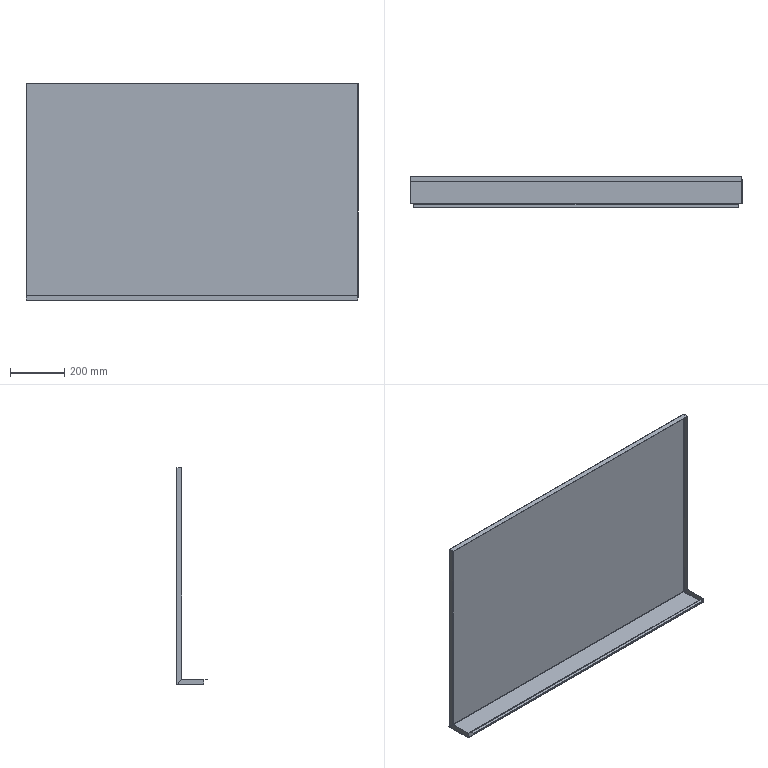Part | SolidWorks | features EdgeFlange 4, FlatPattern 1, ICE 1, SMBaseFlange 1, SheetMetal 1 | 1 solid | 80 faces | box 1220 x 113.8 x 800 mm | volume 1428081 mm3 | plane 56 | cylinder 16 | spline 8 | commonest cylinder face diameters 0.9 x8 3.3 x8